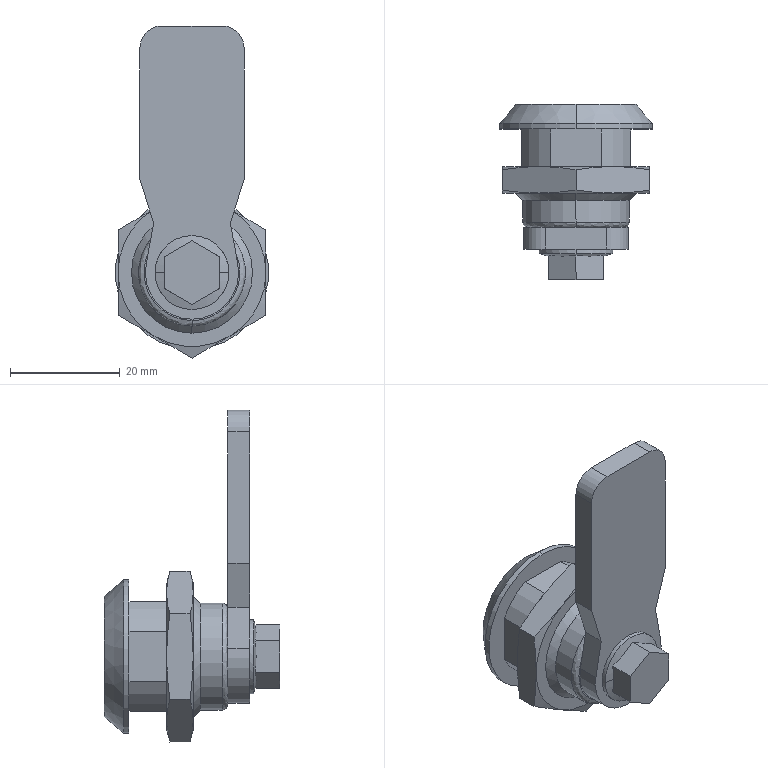Part | SolidWorks | features BaseBody 1 | 1 solid | 87 faces | box 28 x 32 x 60.591 mm | volume 13256 mm3 | plane 39 | cylinder 24 | cone 20 | spline 4 | commonest cylinder face diameters 22 x4 10 x3 16 x3 3 x2 8 x2 13.5 x2